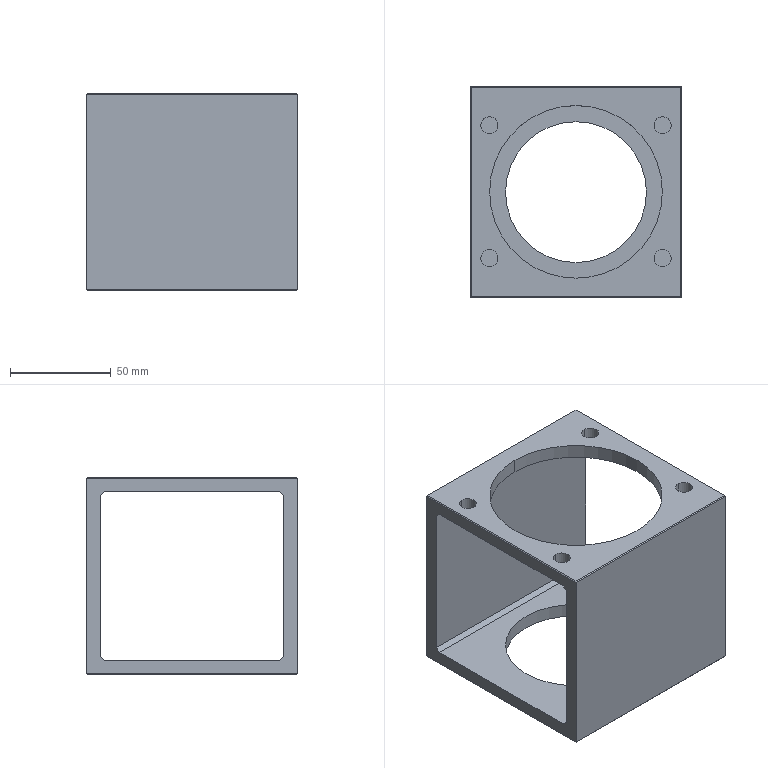Part | Creo | features CURVE 3, DATUM PLANE 3, CHAMFER 2, CUT 2, COORDINATE SYSTEM 1, PROTRUSION 1 | 1 solid | 34 faces | box 105 x 105 x 98 mm | volume 209602 mm3 | plane 22 | cylinder 12 | commonest cylinder face diameters 8.5 x8 70 x2 85.76 x2
STEP:
#1=CARTESIAN_POINT('',(0.,0.,0.));
#2=DIRECTION('',(0.,0.,1.));
#3=DIRECTION('',(1.,0.,0.));
#4=AXIS2_PLACEMENT_3D('',#1,#2,#3);
#5=CARTESIAN_POINT('',(52.,-52.,0.));
#6=VERTEX_POINT('',#5);
#7=CARTESIAN_POINT('',(-52.,-52.,0.));
#8=VERTEX_POINT('',#7);
#9=CARTESIAN_POINT('',(52.,-52.,0.));
#10=DIRECTION('',(-1.,0.,0.));
#11=VECTOR('',#10,104.);
#12=LINE('',#9,#11);
#13=EDGE_CURVE('',#6,#8,#12,.T.);
#14=ORIENTED_EDGE('',*,*,#13,.F.);
#15=CARTESIAN_POINT('',(52.,52.,0.));
#16=VERTEX_POINT('',#15);
#17=CARTESIAN_POINT('',(52.,52.,0.));
#18=DIRECTION('',(0.,-1.,0.));
#19=VECTOR('',#18,104.);
#20=LINE('',#17,#19);
#21=EDGE_CURVE('',#16,#6,#20,.T.);
#22=ORIENTED_EDGE('',*,*,#21,.F.);
#23=CARTESIAN_POINT('',(-52.,52.,0.));
#24=VERTEX_POINT('',#23);
#25=CARTESIAN_POINT('',(-52.,52.,0.));
#26=DIRECTION('',(1.,0.,0.));
#27=VECTOR('',#26,104.);
#28=LINE('',#25,#27);
#29=EDGE_CURVE('',#24,#16,#28,.T.);
#30=ORIENTED_EDGE('',*,*,#29,.F.);
#31=CARTESIAN_POINT('',(-52.,-52.,0.));
#32=DIRECTION('',(0.,1.,0.));
#33=VECTOR('',#32,104.);
#34=LINE('',#31,#33);
#35=EDGE_CURVE('',#8,#24,#34,.T.);
#36=ORIENTED_EDGE('',*,*,#35,.F.);
#37=EDGE_LOOP('',(#14,#22,#30,#36));
#38=FACE_OUTER_BOUND('',#37,.F.);
#39=CARTESIAN_POINT('',(35.,0.,0.));
#40=VERTEX_POINT('',#39);
#41=CARTESIAN_POINT('',(-35.,0.,0.));
#42=VERTEX_POINT('',#41);
#43=CARTESIAN_POINT('',(0.,0.,0.));
#44=DIRECTION('',(0.,0.,-1.));
#45=DIRECTION('',(1.,0.,0.));
#46=AXIS2_PLACEMENT_3D('',#43,#44,#45);
#47=CIRCLE('',#46,35.);
#48=EDGE_CURVE('',#40,#42,#47,.T.);
#49=ORIENTED_EDGE('',*,*,#48,.T.);
#50=CARTESIAN_POINT('',(0.,0.,0.));
#51=DIRECTION('',(0.,0.,-1.));
#52=DIRECTION('',(-1.,0.,0.));
#53=AXIS2_PLACEMENT_3D('',#50,#51,#52);
#54=CIRCLE('',#53,35.);
#55=EDGE_CURVE('',#42,#40,#54,.T.);
#56=ORIENTED_EDGE('',*,*,#55,.T.);
#57=EDGE_LOOP('',(#49,#56));
#58=FACE_BOUND('',#57,.F.);
#59=CARTESIAN_POINT('',(0.,0.,0.));
#60=DIRECTION('',(0.,0.,1.));
#61=DIRECTION('',(1.,0.,0.));
#62=AXIS2_PLACEMENT_3D('',#59,#60,#61);
#63=PLANE('',#62);
#64=ADVANCED_FACE('',(#38,#58),#63,.F.);
#65=CARTESIAN_POINT('',(-35.,0.,7.));
#66=VERTEX_POINT('',#65);
#67=CARTESIAN_POINT('',(35.,0.,7.));
#68=VERTEX_POINT('',#67);
#69=CARTESIAN_POINT('',(0.,0.,7.));
#70=DIRECTION('',(0.,0.,1.));
#71=DIRECTION('',(-1.,0.,0.));
#72=AXIS2_PLACEMENT_3D('',#69,#70,#71);
#73=CIRCLE('',#72,35.);
#74=EDGE_CURVE('',#66,#68,#73,.T.);
#75=ORIENTED_EDGE('',*,*,#74,.F.);
#76=CARTESIAN_POINT('',(-35.,0.,0.));
#77=DIRECTION('',(0.,0.,1.));
#78=VECTOR('',#77,7.);
#79=LINE('',#76,#78);
#80=EDGE_CURVE('',#42,#66,#79,.T.);
#81=ORIENTED_EDGE('',*,*,#80,.F.);
#82=ORIENTED_EDGE('',*,*,#48,.F.);
#83=CARTESIAN_POINT('',(35.,0.,0.));
#84=DIRECTION('',(0.,0.,1.));
#85=VECTOR('',#84,7.);
#86=LINE('',#83,#85);
#87=EDGE_CURVE('',#40,#68,#86,.T.);
#88=ORIENTED_EDGE('',*,*,#87,.T.);
#89=EDGE_LOOP('',(#75,#81,#82,#88));
#90=FACE_OUTER_BOUND('',#89,.F.);
#91=CARTESIAN_POINT('',(0.,0.,0.));
#92=DIRECTION('',(0.,0.,1.));
#93=DIRECTION('',(1.,0.,0.));
#94=AXIS2_PLACEMENT_3D('',#91,#92,#93);
#95=CYLINDRICAL_SURFACE('',#94,35.);
#96=ADVANCED_FACE('',(#90),#95,.F.);
#97=CARTESIAN_POINT('',(52.5,-43.5,7.));
#98=VERTEX_POINT('',#97);
#99=CARTESIAN_POINT('',(-52.5,-43.5,7.));
#100=VERTEX_POINT('',#99);
#101=CARTESIAN_POINT('',(52.5,-43.5,7.));
#102=DIRECTION('',(-1.,0.,0.));
#103=VECTOR('',#102,105.);
#104=LINE('',#101,#103);
#105=EDGE_CURVE('',#98,#100,#104,.T.);
#106=ORIENTED_EDGE('',*,*,#105,.T.);
#107=CARTESIAN_POINT('',(-52.5,43.5,7.));
#108=VERTEX_POINT('',#107);
#109=CARTESIAN_POINT('',(-52.5,-43.5,7.));
#110=DIRECTION('',(0.,1.,0.));
#111=VECTOR('',#110,87.);
#112=LINE('',#109,#111);
#113=EDGE_CURVE('',#100,#108,#112,.T.);
#114=ORIENTED_EDGE('',*,*,#113,.T.);
#115=CARTESIAN_POINT('',(52.5,43.5,7.));
#116=VERTEX_POINT('',#115);
#117=CARTESIAN_POINT('',(52.5,43.5,7.));
#118=DIRECTION('',(-1.,0.,0.));
#119=VECTOR('',#118,105.);
#120=LINE('',#117,#119);
#121=EDGE_CURVE('',#116,#108,#120,.T.);
#122=ORIENTED_EDGE('',*,*,#121,.F.);
#123=CARTESIAN_POINT('',(52.5,-43.5,7.));
#124=DIRECTION('',(0.,1.,0.));
#125=VECTOR('',#124,87.);
#126=LINE('',#123,#125);
#127=EDGE_CURVE('',#98,#116,#126,.T.);
#128=ORIENTED_EDGE('',*,*,#127,.F.);
#129=EDGE_LOOP('',(#106,#114,#122,#128));
#130=FACE_OUTER_BOUND('',#129,.F.);
#131=ORIENTED_EDGE('',*,*,#74,.T.);
#132=CARTESIAN_POINT('',(0.,0.,7.));
#133=DIRECTION('',(0.,0.,1.));
#134=DIRECTION('',(1.,0.,0.));
#135=AXIS2_PLACEMENT_3D('',#132,#133,#134);
#136=CIRCLE('',#135,35.);
#137=EDGE_CURVE('',#68,#66,#136,.T.);
#138=ORIENTED_EDGE('',*,*,#137,.T.);
#139=EDGE_LOOP('',(#131,#138));
#140=FACE_BOUND('',#139,.F.);
#141=CARTESIAN_POINT('',(52.5,-45.5,7.));
#142=DIRECTION('',(0.,0.,-1.));
#143=DIRECTION('',(0.,1.,0.));
#144=AXIS2_PLACEMENT_3D('',#141,#142,#143);
#145=PLANE('',#144);
#146=ADVANCED_FACE('',(#130,#140),#145,.F.);
#147=ORIENTED_EDGE('',*,*,#137,.F.);
#148=ORIENTED_EDGE('',*,*,#87,.F.);
#149=ORIENTED_EDGE('',*,*,#55,.F.);
#150=ORIENTED_EDGE('',*,*,#80,.T.);
#151=EDGE_LOOP('',(#147,#148,#149,#150));
#152=FACE_OUTER_BOUND('',#151,.F.);
#153=CARTESIAN_POINT('',(0.,0.,0.));
#154=DIRECTION('',(0.,0.,1.));
#155=DIRECTION('',(1.,0.,0.));
#156=AXIS2_PLACEMENT_3D('',#153,#154,#155);
#157=CYLINDRICAL_SURFACE('',#156,35.);
#158=ADVANCED_FACE('',(#152),#157,.F.);
#159=ORIENTED_EDGE('',*,*,#105,.F.);
#160=CARTESIAN_POINT('',(52.5,-45.5,9.));
#161=VERTEX_POINT('',#160);
#162=CARTESIAN_POINT('',(52.5,-43.5,7.));
#163=DIRECTION('',(0.,-0.7071,0.7071));
#164=VECTOR('',#163,2.828);
#165=LINE('',#162,#164);
#166=EDGE_CURVE('',#98,#161,#165,.T.);
#167=ORIENTED_EDGE('',*,*,#166,.T.);
#168=CARTESIAN_POINT('',(-52.5,-45.5,9.));
#169=VERTEX_POINT('',#168);
#170=CARTESIAN_POINT('',(52.5,-45.5,9.));
#171=DIRECTION('',(-1.,0.,0.));
#172=VECTOR('',#171,105.);
#173=LINE('',#170,#172);
#174=EDGE_CURVE('',#161,#169,#173,.T.);
#175=ORIENTED_EDGE('',*,*,#174,.T.);
#176=CARTESIAN_POINT('',(-52.5,-45.5,9.));
#177=DIRECTION('',(0.,0.7071,-0.7071));
#178=VECTOR('',#177,2.828);
#179=LINE('',#176,#178);
#180=EDGE_CURVE('',#169,#100,#179,.T.);
#181=ORIENTED_EDGE('',*,*,#180,.T.);
#182=EDGE_LOOP('',(#159,#167,#175,#181));
#183=FACE_OUTER_BOUND('',#182,.F.);
#184=CARTESIAN_POINT('',(0.,-44.5,8.));
#185=DIRECTION('',(0.,0.7071,0.7071));
#186=DIRECTION('',(0.,0.7071,-0.7071));
#187=AXIS2_PLACEMENT_3D('',#184,#185,#186);
#188=PLANE('',#187);
#189=ADVANCED_FACE('',(#183),#188,.T.);
#190=CARTESIAN_POINT('',(52.5,52.5,0.5));
#191=VERTEX_POINT('',#190);
#192=CARTESIAN_POINT('',(52.5,-52.5,0.5));
#193=VERTEX_POINT('',#192);
#194=CARTESIAN_POINT('',(52.5,52.5,0.5));
#195=DIRECTION('',(0.,-1.,0.));
#196=VECTOR('',#195,105.);
#197=LINE('',#194,#196);
#198=EDGE_CURVE('',#191,#193,#197,.T.);
#199=ORIENTED_EDGE('',*,*,#198,.T.);
#200=CARTESIAN_POINT('',(52.5,-52.5,97.5));
#201=VERTEX_POINT('',#200);
#202=CARTESIAN_POINT('',(52.5,-52.5,0.5));
#203=DIRECTION('',(0.,0.,1.));
#204=VECTOR('',#203,97.);
#205=LINE('',#202,#204);
#206=EDGE_CURVE('',#193,#201,#205,.T.);
#207=ORIENTED_EDGE('',*,*,#206,.T.);
#208=CARTESIAN_POINT('',(52.5,52.5,97.5));
#209=VERTEX_POINT('',#208);
#210=CARTESIAN_POINT('',(52.5,-52.5,97.5));
#211=DIRECTION('',(0.,1.,0.));
#212=VECTOR('',#211,105.);
#213=LINE('',#210,#212);
#214=EDGE_CURVE('',#201,#209,#213,.T.);
#215=ORIENTED_EDGE('',*,*,#214,.T.);
#216=CARTESIAN_POINT('',(52.5,52.5,0.5));
#217=DIRECTION('',(0.,0.,1.));
#218=VECTOR('',#217,97.);
#219=LINE('',#216,#218);
#220=EDGE_CURVE('',#191,#209,#219,.T.);
#221=ORIENTED_EDGE('',*,*,#220,.F.);
#222=EDGE_LOOP('',(#199,#207,#215,#221));
#223=FACE_OUTER_BOUND('',#222,.F.);
#224=CARTESIAN_POINT('',(52.5,43.5,91.));
#225=VERTEX_POINT('',#224);
#226=CARTESIAN_POINT('',(52.5,-43.5,91.));
#227=VERTEX_POINT('',#226);
#228=CARTESIAN_POINT('',(52.5,43.5,91.));
#229=DIRECTION('',(0.,-1.,0.));
#230=VECTOR('',#229,87.);
#231=LINE('',#228,#230);
#232=EDGE_CURVE('',#225,#227,#231,.T.);
#233=ORIENTED_EDGE('',*,*,#232,.T.);
#234=CARTESIAN_POINT('',(52.5,-45.5,89.));
#235=VERTEX_POINT('',#234);
#236=CARTESIAN_POINT('',(52.5,-45.5,89.));
#237=DIRECTION('',(0.,0.7071,0.7071));
#238=VECTOR('',#237,2.828);
#239=LINE('',#236,#238);
#240=EDGE_CURVE('',#235,#227,#239,.T.);
#241=ORIENTED_EDGE('',*,*,#240,.F.);
#242=CARTESIAN_POINT('',(52.5,-45.5,89.));
#243=DIRECTION('',(0.,0.,-1.));
#244=VECTOR('',#243,80.);
#245=LINE('',#242,#244);
#246=EDGE_CURVE('',#235,#161,#245,.T.);
#247=ORIENTED_EDGE('',*,*,#246,.T.);
#248=ORIENTED_EDGE('',*,*,#166,.F.);
#249=ORIENTED_EDGE('',*,*,#127,.T.);
#250=CARTESIAN_POINT('',(52.5,45.5,9.));
#251=VERTEX_POINT('',#250);
#252=CARTESIAN_POINT('',(52.5,45.5,9.));
#253=DIRECTION('',(0.,-0.7071,-0.7071));
#254=VECTOR('',#253,2.828);
#255=LINE('',#252,#254);
#256=EDGE_CURVE('',#251,#116,#255,.T.);
#257=ORIENTED_EDGE('',*,*,#256,.F.);
#258=CARTESIAN_POINT('',(52.5,45.5,89.));
#259=VERTEX_POINT('',#258);
#260=CARTESIAN_POINT('',(52.5,45.5,9.));
#261=DIRECTION('',(0.,0.,1.));
#262=VECTOR('',#261,80.);
#263=LINE('',#260,#262);
#264=EDGE_CURVE('',#251,#259,#263,.T.);
#265=ORIENTED_EDGE('',*,*,#264,.T.);
#266=CARTESIAN_POINT('',(52.5,43.5,91.));
#267=DIRECTION('',(0.,0.7071,-0.7071));
#268=VECTOR('',#267,2.828);
#269=LINE('',#266,#268);
#270=EDGE_CURVE('',#225,#259,#269,.T.);
#271=ORIENTED_EDGE('',*,*,#270,.F.);
#272=EDGE_LOOP('',(#233,#241,#247,#248,#249,#257,#265,#271));
#273=FACE_BOUND('',#272,.F.);
#274=CARTESIAN_POINT('',(52.5,-52.5,0.));
#275=DIRECTION('',(1.,0.,0.));
#276=DIRECTION('',(0.,1.,0.));
#277=AXIS2_PLACEMENT_3D('',#274,#275,#276);
#278=PLANE('',#277);
#279=ADVANCED_FACE('',(#223,#273),#278,.T.);
#280=CARTESIAN_POINT('',(-52.5,43.5,91.));
#281=VERTEX_POINT('',#280);
#282=CARTESIAN_POINT('',(52.5,43.5,91.));
#283=DIRECTION('',(-1.,0.,0.));
#284=VECTOR('',#283,105.);
#285=LINE('',#282,#284);
#286=EDGE_CURVE('',#225,#281,#285,.T.);
#287=ORIENTED_EDGE('',*,*,#286,.T.);
#288=CARTESIAN_POINT('',(-52.5,-43.5,91.));
#289=VERTEX_POINT('',#288);
#290=CARTESIAN_POINT('',(-52.5,43.5,91.));
#291=DIRECTION('',(0.,-1.,0.));
#292=VECTOR('',#291,87.);
#293=LINE('',#290,#292);
#294=EDGE_CURVE('',#281,#289,#293,.T.);
#295=ORIENTED_EDGE('',*,*,#294,.T.);
#296=CARTESIAN_POINT('',(52.5,-43.5,91.));
#297=DIRECTION('',(-1.,0.,0.));
#298=VECTOR('',#297,105.);
#299=LINE('',#296,#298);
#300=EDGE_CURVE('',#227,#289,#299,.T.);
#301=ORIENTED_EDGE('',*,*,#300,.F.);
#302=ORIENTED_EDGE('',*,*,#232,.F.);
#303=EDGE_LOOP('',(#287,#295,#301,#302));
#304=FACE_OUTER_BOUND('',#303,.F.);
#305=CARTESIAN_POINT('',(-43.,37.25,91.));
#306=VERTEX_POINT('',#305);
#307=CARTESIAN_POINT('',(-43.,28.75,91.));
#308=VERTEX_POINT('',#307);
#309=CARTESIAN_POINT('',(-43.,33.,91.));
#310=DIRECTION('',(0.,0.,1.));
#311=DIRECTION('',(0.,1.,0.));
#312=AXIS2_PLACEMENT_3D('',#309,#310,#311);
#313=CIRCLE('',#312,4.25);
#314=EDGE_CURVE('',#306,#308,#313,.T.);
#315=ORIENTED_EDGE('',*,*,#314,.F.);
#316=CARTESIAN_POINT('',(-43.,33.,91.));
#317=DIRECTION('',(0.,0.,1.));
#318=DIRECTION('',(0.,-1.,0.));
#319=AXIS2_PLACEMENT_3D('',#316,#317,#318);
#320=CIRCLE('',#319,4.25);
#321=EDGE_CURVE('',#308,#306,#320,.T.);
#322=ORIENTED_EDGE('',*,*,#321,.F.);
#323=EDGE_LOOP('',(#315,#322));
#324=FACE_BOUND('',#323,.F.);
#325=CARTESIAN_POINT('',(-43.,-28.75,91.));
#326=VERTEX_POINT('',#325);
#327=CARTESIAN_POINT('',(-43.,-37.25,91.));
#328=VERTEX_POINT('',#327);
#329=CARTESIAN_POINT('',(-43.,-33.,91.));
#330=DIRECTION('',(0.,0.,1.));
#331=DIRECTION('',(0.,1.,0.));
#332=AXIS2_PLACEMENT_3D('',#329,#330,#331);
#333=CIRCLE('',#332,4.25);
#334=EDGE_CURVE('',#326,#328,#333,.T.);
#335=ORIENTED_EDGE('',*,*,#334,.F.);
#336=CARTESIAN_POINT('',(-43.,-33.,91.));
#337=DIRECTION('',(0.,0.,1.));
#338=DIRECTION('',(0.,-1.,0.));
#339=AXIS2_PLACEMENT_3D('',#336,#337,#338);
#340=CIRCLE('',#339,4.25);
#341=EDGE_CURVE('',#328,#326,#340,.T.);
#342=ORIENTED_EDGE('',*,*,#341,.F.);
#343=EDGE_LOOP('',(#335,#342));
#344=FACE_BOUND('',#343,.F.);
#345=CARTESIAN_POINT('',(43.,-28.75,91.));
#346=VERTEX_POINT('',#345);
#347=CARTESIAN_POINT('',(43.,-37.25,91.));
#348=VERTEX_POINT('',#347);
#349=CARTESIAN_POINT('',(43.,-33.,91.));
#350=DIRECTION('',(0.,0.,1.));
#351=DIRECTION('',(0.,1.,0.));
#352=AXIS2_PLACEMENT_3D('',#349,#350,#351);
#353=CIRCLE('',#352,4.25);
#354=EDGE_CURVE('',#346,#348,#353,.T.);
#355=ORIENTED_EDGE('',*,*,#354,.F.);
#356=CARTESIAN_POINT('',(43.,-33.,91.));
#357=DIRECTION('',(0.,0.,1.));
#358=DIRECTION('',(0.,-1.,0.));
#359=AXIS2_PLACEMENT_3D('',#356,#357,#358);
#360=CIRCLE('',#359,4.25);
#361=EDGE_CURVE('',#348,#346,#360,.T.);
#362=ORIENTED_EDGE('',*,*,#361,.F.);
#363=EDGE_LOOP('',(#355,#362));
#364=FACE_BOUND('',#363,.F.);
#365=CARTESIAN_POINT('',(43.,37.25,91.));
#366=VERTEX_POINT('',#365);
#367=CARTESIAN_POINT('',(43.,28.75,91.));
#368=VERTEX_POINT('',#367);
#369=CARTESIAN_POINT('',(43.,33.,91.));
#370=DIRECTION('',(0.,0.,1.));
#371=DIRECTION('',(0.,1.,0.));
#372=AXIS2_PLACEMENT_3D('',#369,#370,#371);
#373=CIRCLE('',#372,4.25);
#374=EDGE_CURVE('',#366,#368,#373,.T.);
#375=ORIENTED_EDGE('',*,*,#374,.F.);
#376=CARTESIAN_POINT('',(43.,33.,91.));
#377=DIRECTION('',(0.,0.,1.));
#378=DIRECTION('',(0.,-1.,0.));
#379=AXIS2_PLACEMENT_3D('',#376,#377,#378);
#380=CIRCLE('',#379,4.25);
#381=EDGE_CURVE('',#368,#366,#380,.T.);
#382=ORIENTED_EDGE('',*,*,#381,.F.);
#383=EDGE_LOOP('',(#375,#382));
#384=FACE_BOUND('',#383,.F.);
#385=CARTESIAN_POINT('',(0.,42.88,91.));
#386=VERTEX_POINT('',#385);
#387=CARTESIAN_POINT('',(0.,-42.88,91.));
#388=VERTEX_POINT('',#387);
#389=CARTESIAN_POINT('',(0.,0.,91.));
#390=DIRECTION('',(0.,0.,1.));
#391=DIRECTION('',(0.,1.,0.));
#392=AXIS2_PLACEMENT_3D('',#389,#390,#391);
#393=CIRCLE('',#392,42.88);
#394=EDGE_CURVE('',#386,#388,#393,.T.);
#395=ORIENTED_EDGE('',*,*,#394,.F.);
#396=CARTESIAN_POINT('',(0.,0.,91.));
#397=DIRECTION('',(0.,0.,1.));
#398=DIRECTION('',(0.,-1.,0.));
#399=AXIS2_PLACEMENT_3D('',#396,#397,#398);
#400=CIRCLE('',#399,42.88);
#401=EDGE_CURVE('',#388,#386,#400,.T.);
#402=ORIENTED_EDGE('',*,*,#401,.F.);
#403=EDGE_LOOP('',(#395,#402));
#404=FACE_BOUND('',#403,.F.);
#405=CARTESIAN_POINT('',(52.5,45.5,91.));
#406=DIRECTION('',(0.,0.,1.));
#407=DIRECTION('',(0.,-1.,0.));
#408=AXIS2_PLACEMENT_3D('',#405,#406,#407);
#409=PLANE('',#408);
#410=ADVANCED_FACE('',(#304,#324,#344,#364,#384,#404),#409,.F.);
#411=CARTESIAN_POINT('',(0.,42.88,98.));
#412=VERTEX_POINT('',#411);
#413=CARTESIAN_POINT('',(0.,-42.88,98.));
#414=VERTEX_POINT('',#413);
#415=CARTESIAN_POINT('',(0.,0.,98.));
#416=DIRECTION('',(0.,0.,1.));
#417=DIRECTION('',(0.,1.,0.));
#418=AXIS2_PLACEMENT_3D('',#415,#416,#417);
#419=CIRCLE('',#418,42.88);
#420=EDGE_CURVE('',#412,#414,#419,.T.);
#421=ORIENTED_EDGE('',*,*,#420,.F.);
#422=CARTESIAN_POINT('',(0.,42.88,98.));
#423=DIRECTION('',(0.,0.,-1.));
#424=VECTOR('',#423,7.);
#425=LINE('',#422,#424);
#426=EDGE_CURVE('',#412,#386,#425,.T.);
#427=ORIENTED_EDGE('',*,*,#426,.T.);
#428=ORIENTED_EDGE('',*,*,#394,.T.);
#429=CARTESIAN_POINT('',(0.,-42.88,98.));
#430=DIRECTION('',(0.,0.,-1.));
#431=VECTOR('',#430,7.);
#432=LINE('',#429,#431);
#433=EDGE_CURVE('',#414,#388,#432,.T.);
#434=ORIENTED_EDGE('',*,*,#433,.F.);
#435=EDGE_LOOP('',(#421,#427,#428,#434));
#436=FACE_OUTER_BOUND('',#435,.F.);
#437=CARTESIAN_POINT('',(0.,0.,98.));
#438=DIRECTION('',(0.,0.,1.));
#439=DIRECTION('',(0.,1.,0.));
#440=AXIS2_PLACEMENT_3D('',#437,#438,#439);
#441=CYLINDRICAL_SURFACE('',#440,42.88);
#442=ADVANCED_FACE('',(#436),#441,.F.);
#443=CARTESIAN_POINT('',(-52.,52.,98.));
#444=VERTEX_POINT('',#443);
#445=CARTESIAN_POINT('',(-52.,-52.,98.));
#446=VERTEX_POINT('',#445);
#447=CARTESIAN_POINT('',(-52.,52.,98.));
#448=DIRECTION('',(0.,-1.,0.));
#449=VECTOR('',#448,104.);
#450=LINE('',#447,#449);
#451=EDGE_CURVE('',#444,#446,#450,.T.);
#452=ORIENTED_EDGE('',*,*,#451,.F.);
#453=CARTESIAN_POINT('',(52.,52.,98.));
#454=VERTEX_POINT('',#453);
#455=CARTESIAN_POINT('',(52.,52.,98.));
#456=DIRECTION('',(-1.,0.,0.));
#457=VECTOR('',#456,104.);
#458=LINE('',#455,#457);
#459=EDGE_CURVE('',#454,#444,#458,.T.);
#460=ORIENTED_EDGE('',*,*,#459,.F.);
#461=CARTESIAN_POINT('',(52.,-52.,98.));
#462=VERTEX_POINT('',#461);
#463=CARTESIAN_POINT('',(52.,-52.,98.));
#464=DIRECTION('',(0.,1.,0.));
#465=VECTOR('',#464,104.);
#466=LINE('',#463,#465);
#467=EDGE_CURVE('',#462,#454,#466,.T.);
#468=ORIENTED_EDGE('',*,*,#467,.F.);
#469=CARTESIAN_POINT('',(-52.,-52.,98.));
#470=DIRECTION('',(1.,0.,0.));
#471=VECTOR('',#470,104.);
#472=LINE('',#469,#471);
#473=EDGE_CURVE('',#446,#462,#472,.T.);
#474=ORIENTED_EDGE('',*,*,#473,.F.);
#475=EDGE_LOOP('',(#452,#460,#468,#474));
#476=FACE_OUTER_BOUND('',#475,.F.);
#477=CARTESIAN_POINT('',(-43.,37.25,98.));
#478=VERTEX_POINT('',#477);
#479=CARTESIAN_POINT('',(-43.,28.75,98.));
#480=VERTEX_POINT('',#479);
#481=CARTESIAN_POINT('',(-43.,33.,98.));
#482=DIRECTION('',(0.,0.,1.));
#483=DIRECTION('',(0.,1.,0.));
#484=AXIS2_PLACEMENT_3D('',#481,#482,#483);
#485=CIRCLE('',#484,4.25);
#486=EDGE_CURVE('',#478,#480,#485,.T.);
#487=ORIENTED_EDGE('',*,*,#486,.T.);
#488=CARTESIAN_POINT('',(-43.,33.,98.));
#489=DIRECTION('',(0.,0.,1.));
#490=DIRECTION('',(0.,-1.,0.));
#491=AXIS2_PLACEMENT_3D('',#488,#489,#490);
#492=CIRCLE('',#491,4.25);
#493=EDGE_CURVE('',#480,#478,#492,.T.);
#494=ORIENTED_EDGE('',*,*,#493,.T.);
#495=EDGE_LOOP('',(#487,#494));
#496=FACE_BOUND('',#495,.F.);
#497=CARTESIAN_POINT('',(-43.,-28.75,98.));
#498=VERTEX_POINT('',#497);
#499=CARTESIAN_POINT('',(-43.,-37.25,98.));
#500=VERTEX_POINT('',#499);
#501=CARTESIAN_POINT('',(-43.,-33.,98.));
#502=DIRECTION('',(0.,0.,1.));
#503=DIRECTION('',(0.,1.,0.));
#504=AXIS2_PLACEMENT_3D('',#501,#502,#503);
#505=CIRCLE('',#504,4.25);
#506=EDGE_CURVE('',#498,#500,#505,.T.);
#507=ORIENTED_EDGE('',*,*,#506,.T.);
#508=CARTESIAN_POINT('',(-43.,-33.,98.));
#509=DIRECTION('',(0.,0.,1.));
#510=DIRECTION('',(0.,-1.,0.));
#511=AXIS2_PLACEMENT_3D('',#508,#509,#510);
#512=CIRCLE('',#511,4.25);
#513=EDGE_CURVE('',#500,#498,#512,.T.);
#514=ORIENTED_EDGE('',*,*,#513,.T.);
#515=EDGE_LOOP('',(#507,#514));
#516=FACE_BOUND('',#515,.F.);
#517=CARTESIAN_POINT('',(43.,-28.75,98.));
#518=VERTEX_POINT('',#517);
#519=CARTESIAN_POINT('',(43.,-37.25,98.));
#520=VERTEX_POINT('',#519);
#521=CARTESIAN_POINT('',(43.,-33.,98.));
#522=DIRECTION('',(0.,0.,1.));
#523=DIRECTION('',(0.,1.,0.));
#524=AXIS2_PLACEMENT_3D('',#521,#522,#523);
#525=CIRCLE('',#524,4.25);
#526=EDGE_CURVE('',#518,#520,#525,.T.);
#527=ORIENTED_EDGE('',*,*,#526,.T.);
#528=CARTESIAN_POINT('',(43.,-33.,98.));
#529=DIRECTION('',(0.,0.,1.));
#530=DIRECTION('',(0.,-1.,0.));
#531=AXIS2_PLACEMENT_3D('',#528,#529,#530);
#532=CIRCLE('',#531,4.25);
#533=EDGE_CURVE('',#520,#518,#532,.T.);
#534=ORIENTED_EDGE('',*,*,#533,.T.);
#535=EDGE_LOOP('',(#527,#534));
#536=FACE_BOUND('',#535,.F.);
#537=CARTESIAN_POINT('',(43.,37.25,98.));
#538=VERTEX_POINT('',#537);
#539=CARTESIAN_POINT('',(43.,28.75,98.));
#540=VERTEX_POINT('',#539);
#541=CARTESIAN_POINT('',(43.,33.,98.));
#542=DIRECTION('',(0.,0.,1.));
#543=DIRECTION('',(0.,1.,0.));
#544=AXIS2_PLACEMENT_3D('',#541,#542,#543);
#545=CIRCLE('',#544,4.25);
#546=EDGE_CURVE('',#538,#540,#545,.T.);
#547=ORIENTED_EDGE('',*,*,#546,.T.);
#548=CARTESIAN_POINT('',(43.,33.,98.));
#549=DIRECTION('',(0.,0.,1.));
#550=DIRECTION('',(0.,-1.,0.));
#551=AXIS2_PLACEMENT_3D('',#548,#549,#550);
#552=CIRCLE('',#551,4.25);
#553=EDGE_CURVE('',#540,#538,#552,.T.);
#554=ORIENTED_EDGE('',*,*,#553,.T.);
#555=EDGE_LOOP('',(#547,#554));
#556=FACE_BOUND('',#555,.F.);
#557=ORIENTED_EDGE('',*,*,#420,.T.);
#558=CARTESIAN_POINT('',(0.,0.,98.));
#559=DIRECTION('',(0.,0.,1.));
#560=DIRECTION('',(0.,-1.,0.));
#561=AXIS2_PLACEMENT_3D('',#558,#559,#560);
#562=CIRCLE('',#561,42.88);
#563=EDGE_CURVE('',#414,#412,#562,.T.);
#564=ORIENTED_EDGE('',*,*,#563,.T.);
#565=EDGE_LOOP('',(#557,#564));
#566=FACE_BOUND('',#565,.F.);
#567=CARTESIAN_POINT('',(0.,0.,98.));
#568=DIRECTION('',(0.,0.,1.));
#569=DIRECTION('',(1.,0.,0.));
#570=AXIS2_PLACEMENT_3D('',#567,#568,#569);
#571=PLANE('',#570);
#572=ADVANCED_FACE('',(#476,#496,#516,#536,#556,#566),#571,.T.);
#573=ORIENTED_EDGE('',*,*,#563,.F.);
#574=ORIENTED_EDGE('',*,*,#433,.T.);
#575=ORIENTED_EDGE('',*,*,#401,.T.);
#576=ORIENTED_EDGE('',*,*,#426,.F.);
#577=EDGE_LOOP('',(#573,#574,#575,#576));
#578=FACE_OUTER_BOUND('',#577,.F.);
#579=CARTESIAN_POINT('',(0.,0.,98.));
#580=DIRECTION('',(0.,0.,1.));
#581=DIRECTION('',(0.,1.,0.));
#582=AXIS2_PLACEMENT_3D('',#579,#580,#581);
#583=CYLINDRICAL_SURFACE('',#582,42.88);
#584=ADVANCED_FACE('',(#578),#583,.F.);
#585=ORIENTED_EDGE('',*,*,#486,.F.);
#586=CARTESIAN_POINT('',(-43.,37.25,98.));
#587=DIRECTION('',(0.,0.,-1.));
#588=VECTOR('',#587,7.);
#589=LINE('',#586,#588);
#590=EDGE_CURVE('',#478,#306,#589,.T.);
#591=ORIENTED_EDGE('',*,*,#590,.T.);
#592=ORIENTED_EDGE('',*,*,#314,.T.);
#593=CARTESIAN_POINT('',(-43.,28.75,98.));
#594=DIRECTION('',(0.,0.,-1.));
#595=VECTOR('',#594,7.);
#596=LINE('',#593,#595);
#597=EDGE_CURVE('',#480,#308,#596,.T.);
#598=ORIENTED_EDGE('',*,*,#597,.F.);
#599=EDGE_LOOP('',(#585,#591,#592,#598));
#600=FACE_OUTER_BOUND('',#599,.F.);
#601=CARTESIAN_POINT('',(-43.,33.,98.));
#602=DIRECTION('',(0.,0.,1.));
#603=DIRECTION('',(0.,1.,0.));
#604=AXIS2_PLACEMENT_3D('',#601,#602,#603);
#605=CYLINDRICAL_SURFACE('',#604,4.25);
#606=ADVANCED_FACE('',(#600),#605,.F.);
#607=ORIENTED_EDGE('',*,*,#493,.F.);
#608=ORIENTED_EDGE('',*,*,#597,.T.);
#609=ORIENTED_EDGE('',*,*,#321,.T.);
#610=ORIENTED_EDGE('',*,*,#590,.F.);
#611=EDGE_LOOP('',(#607,#608,#609,#610));
#612=FACE_OUTER_BOUND('',#611,.F.);
#613=CARTESIAN_POINT('',(-43.,33.,98.));
#614=DIRECTION('',(0.,0.,1.));
#615=DIRECTION('',(0.,1.,0.));
#616=AXIS2_PLACEMENT_3D('',#613,#614,#615);
#617=CYLINDRICAL_SURFACE('',#616,4.25);
#618=ADVANCED_FACE('',(#612),#617,.F.);
#619=ORIENTED_EDGE('',*,*,#506,.F.);
#620=CARTESIAN_POINT('',(-43.,-28.75,98.));
#621=DIRECTION('',(0.,0.,-1.));
#622=VECTOR('',#621,7.);
#623=LINE('',#620,#622);
#624=EDGE_CURVE('',#498,#326,#623,.T.);
#625=ORIENTED_EDGE('',*,*,#624,.T.);
#626=ORIENTED_EDGE('',*,*,#334,.T.);
#627=CARTESIAN_POINT('',(-43.,-37.25,98.));
#628=DIRECTION('',(0.,0.,-1.));
#629=VECTOR('',#628,7.);
#630=LINE('',#627,#629);
#631=EDGE_CURVE('',#500,#328,#630,.T.);
#632=ORIENTED_EDGE('',*,*,#631,.F.);
#633=EDGE_LOOP('',(#619,#625,#626,#632));
#634=FACE_OUTER_BOUND('',#633,.F.);
#635=CARTESIAN_POINT('',(-43.,-33.,98.));
#636=DIRECTION('',(0.,0.,1.));
#637=DIRECTION('',(0.,1.,0.));
#638=AXIS2_PLACEMENT_3D('',#635,#636,#637);
#639=CYLINDRICAL_SURFACE('',#638,4.25);
#640=ADVANCED_FACE('',(#634),#639,.F.);
#641=ORIENTED_EDGE('',*,*,#513,.F.);
#642=ORIENTED_EDGE('',*,*,#631,.T.);
#643=ORIENTED_EDGE('',*,*,#341,.T.);
#644=ORIENTED_EDGE('',*,*,#624,.F.);
#645=EDGE_LOOP('',(#641,#642,#643,#644));
#646=FACE_OUTER_BOUND('',#645,.F.);
#647=CARTESIAN_POINT('',(-43.,-33.,98.));
#648=DIRECTION('',(0.,0.,1.));
#649=DIRECTION('',(0.,1.,0.));
#650=AXIS2_PLACEMENT_3D('',#647,#648,#649);
#651=CYLINDRICAL_SURFACE('',#650,4.25);
#652=ADVANCED_FACE('',(#646),#651,.F.);
#653=ORIENTED_EDGE('',*,*,#526,.F.);
#654=CARTESIAN_POINT('',(43.,-28.75,98.));
#655=DIRECTION('',(0.,0.,-1.));
#656=VECTOR('',#655,7.);
#657=LINE('',#654,#656);
#658=EDGE_CURVE('',#518,#346,#657,.T.);
#659=ORIENTED_EDGE('',*,*,#658,.T.);
#660=ORIENTED_EDGE('',*,*,#354,.T.);
#661=CARTESIAN_POINT('',(43.,-37.25,98.));
#662=DIRECTION('',(0.,0.,-1.));
#663=VECTOR('',#662,7.);
#664=LINE('',#661,#663);
#665=EDGE_CURVE('',#520,#348,#664,.T.);
#666=ORIENTED_EDGE('',*,*,#665,.F.);
#667=EDGE_LOOP('',(#653,#659,#660,#666));
#668=FACE_OUTER_BOUND('',#667,.F.);
#669=CARTESIAN_POINT('',(43.,-33.,98.));
#670=DIRECTION('',(0.,0.,1.));
#671=DIRECTION('',(0.,1.,0.));
#672=AXIS2_PLACEMENT_3D('',#669,#670,#671);
#673=CYLINDRICAL_SURFACE('',#672,4.25);
#674=ADVANCED_FACE('',(#668),#673,.F.);
#675=ORIENTED_EDGE('',*,*,#533,.F.);
#676=ORIENTED_EDGE('',*,*,#665,.T.);
#677=ORIENTED_EDGE('',*,*,#361,.T.);
#678=ORIENTED_EDGE('',*,*,#658,.F.);
#679=EDGE_LOOP('',(#675,#676,#677,#678));
#680=FACE_OUTER_BOUND('',#679,.F.);
#681=CARTESIAN_POINT('',(43.,-33.,98.));
#682=DIRECTION('',(0.,0.,1.));
#683=DIRECTION('',(0.,1.,0.));
#684=AXIS2_PLACEMENT_3D('',#681,#682,#683);
#685=CYLINDRICAL_SURFACE('',#684,4.25);
#686=ADVANCED_FACE('',(#680),#685,.F.);
#687=ORIENTED_EDGE('',*,*,#546,.F.);
#688=CARTESIAN_POINT('',(43.,37.25,98.));
#689=DIRECTION('',(0.,0.,-1.));
#690=VECTOR('',#689,7.);
#691=LINE('',#688,#690);
#692=EDGE_CURVE('',#538,#366,#691,.T.);
#693=ORIENTED_EDGE('',*,*,#692,.T.);
#694=ORIENTED_EDGE('',*,*,#374,.T.);
#695=CARTESIAN_POINT('',(43.,28.75,98.));
#696=DIRECTION('',(0.,0.,-1.));
#697=VECTOR('',#696,7.);
#698=LINE('',#695,#697);
#699=EDGE_CURVE('',#540,#368,#698,.T.);
#700=ORIENTED_EDGE('',*,*,#699,.F.);
#701=EDGE_LOOP('',(#687,#693,#694,#700));
#702=FACE_OUTER_BOUND('',#701,.F.);
#703=CARTESIAN_POINT('',(43.,33.,98.));
#704=DIRECTION('',(0.,0.,1.));
#705=DIRECTION('',(0.,1.,0.));
#706=AXIS2_PLACEMENT_3D('',#703,#704,#705);
#707=CYLINDRICAL_SURFACE('',#706,4.25);
#708=ADVANCED_FACE('',(#702),#707,.F.);
#709=ORIENTED_EDGE('',*,*,#553,.F.);
#710=ORIENTED_EDGE('',*,*,#699,.T.);
#711=ORIENTED_EDGE('',*,*,#381,.T.);
#712=ORIENTED_EDGE('',*,*,#692,.F.);
#713=EDGE_LOOP('',(#709,#710,#711,#712));
#714=FACE_OUTER_BOUND('',#713,.F.);
#715=CARTESIAN_POINT('',(43.,33.,98.));
#716=DIRECTION('',(0.,0.,1.));
#717=DIRECTION('',(0.,1.,0.));
#718=AXIS2_PLACEMENT_3D('',#715,#716,#717);
#719=CYLINDRICAL_SURFACE('',#718,4.25);
#720=ADVANCED_FACE('',(#714),#719,.F.);
#721=CARTESIAN_POINT('',(-52.5,52.5,97.5));
#722=VERTEX_POINT('',#721);
#723=CARTESIAN_POINT('',(-52.5,-52.5,97.5));
#724=VERTEX_POINT('',#723);
#725=CARTESIAN_POINT('',(-52.5,52.5,97.5));
#726=DIRECTION('',(0.,-1.,0.));
#727=VECTOR('',#726,105.);
#728=LINE('',#725,#727);
#729=EDGE_CURVE('',#722,#724,#728,.T.);
#730=ORIENTED_EDGE('',*,*,#729,.F.);
#731=CARTESIAN_POINT('',(-52.5,52.5,97.5));
#732=DIRECTION('',(0.5774,-0.5774,0.5774));
#733=VECTOR('',#732,0.866);
#734=LINE('',#731,#733);
#735=EDGE_CURVE('',#722,#444,#734,.T.);
#736=ORIENTED_EDGE('',*,*,#735,.T.);
#737=ORIENTED_EDGE('',*,*,#451,.T.);
#738=CARTESIAN_POINT('',(-52.5,-52.5,97.5));
#739=DIRECTION('',(0.5774,0.5774,0.5774));
#740=VECTOR('',#739,0.866);
#741=LINE('',#738,#740);
#742=EDGE_CURVE('',#724,#446,#741,.T.);
#743=ORIENTED_EDGE('',*,*,#742,.F.);
#744=EDGE_LOOP('',(#730,#736,#737,#743));
#745=FACE_OUTER_BOUND('',#744,.F.);
#746=CARTESIAN_POINT('',(-52.25,0.,97.75));
#747=DIRECTION('',(-0.7071,0.,0.7071));
#748=DIRECTION('',(-0.7071,0.,-0.7071));
#749=AXIS2_PLACEMENT_3D('',#746,#747,#748);
#750=PLANE('',#749);
#751=ADVANCED_FACE('',(#745),#750,.T.);
#752=CARTESIAN_POINT('',(-52.5,-52.5,0.5));
#753=VERTEX_POINT('',#752);
#754=CARTESIAN_POINT('',(-52.5,52.5,0.5));
#755=VERTEX_POINT('',#754);
#756=CARTESIAN_POINT('',(-52.5,-52.5,0.5));
#757=DIRECTION('',(0.,1.,0.));
#758=VECTOR('',#757,105.);
#759=LINE('',#756,#758);
#760=EDGE_CURVE('',#753,#755,#759,.T.);
#761=ORIENTED_EDGE('',*,*,#760,.T.);
#762=CARTESIAN_POINT('',(-52.5,52.5,0.5));
#763=DIRECTION('',(0.,0.,1.));
#764=VECTOR('',#763,97.);
#765=LINE('',#762,#764);
#766=EDGE_CURVE('',#755,#722,#765,.T.);
#767=ORIENTED_EDGE('',*,*,#766,.T.);
#768=ORIENTED_EDGE('',*,*,#729,.T.);
#769=CARTESIAN_POINT('',(-52.5,-52.5,0.5));
#770=DIRECTION('',(0.,0.,1.));
#771=VECTOR('',#770,97.);
#772=LINE('',#769,#771);
#773=EDGE_CURVE('',#753,#724,#772,.T.);
#774=ORIENTED_EDGE('',*,*,#773,.F.);
#775=EDGE_LOOP('',(#761,#767,#768,#774));
#776=FACE_OUTER_BOUND('',#775,.F.);
#777=CARTESIAN_POINT('',(-52.5,-45.5,89.));
#778=VERTEX_POINT('',#777);
#779=CARTESIAN_POINT('',(-52.5,-45.5,89.));
#780=DIRECTION('',(0.,0.,-1.));
#781=VECTOR('',#780,80.);
#782=LINE('',#779,#781);
#783=EDGE_CURVE('',#778,#169,#782,.T.);
#784=ORIENTED_EDGE('',*,*,#783,.F.);
#785=CARTESIAN_POINT('',(-52.5,-43.5,91.));
#786=DIRECTION('',(0.,-0.7071,-0.7071));
#787=VECTOR('',#786,2.828);
#788=LINE('',#785,#787);
#789=EDGE_CURVE('',#289,#778,#788,.T.);
#790=ORIENTED_EDGE('',*,*,#789,.F.);
#791=ORIENTED_EDGE('',*,*,#294,.F.);
#792=CARTESIAN_POINT('',(-52.5,45.5,89.));
#793=VERTEX_POINT('',#792);
#794=CARTESIAN_POINT('',(-52.5,45.5,89.));
#795=DIRECTION('',(0.,-0.7071,0.7071));
#796=VECTOR('',#795,2.828);
#797=LINE('',#794,#796);
#798=EDGE_CURVE('',#793,#281,#797,.T.);
#799=ORIENTED_EDGE('',*,*,#798,.F.);
#800=CARTESIAN_POINT('',(-52.5,45.5,9.));
#801=VERTEX_POINT('',#800);
#802=CARTESIAN_POINT('',(-52.5,45.5,9.));
#803=DIRECTION('',(0.,0.,1.));
#804=VECTOR('',#803,80.);
#805=LINE('',#802,#804);
#806=EDGE_CURVE('',#801,#793,#805,.T.);
#807=ORIENTED_EDGE('',*,*,#806,.F.);
#808=CARTESIAN_POINT('',(-52.5,43.5,7.));
#809=DIRECTION('',(0.,0.7071,0.7071));
#810=VECTOR('',#809,2.828);
#811=LINE('',#808,#810);
#812=EDGE_CURVE('',#108,#801,#811,.T.);
#813=ORIENTED_EDGE('',*,*,#812,.F.);
#814=ORIENTED_EDGE('',*,*,#113,.F.);
#815=ORIENTED_EDGE('',*,*,#180,.F.);
#816=EDGE_LOOP('',(#784,#790,#791,#799,#807,#813,#814,#815));
#817=FACE_BOUND('',#816,.F.);
#818=CARTESIAN_POINT('',(-52.5,52.5,0.));
#819=DIRECTION('',(-1.,0.,0.));
#820=DIRECTION('',(0.,-1.,0.));
#821=AXIS2_PLACEMENT_3D('',#818,#819,#820);
#822=PLANE('',#821);
#823=ADVANCED_FACE('',(#776,#817),#822,.T.);
#824=CARTESIAN_POINT('',(52.5,-45.5,89.));
#825=DIRECTION('',(-1.,0.,0.));
#826=VECTOR('',#825,105.);
#827=LINE('',#824,#826);
#828=EDGE_CURVE('',#235,#778,#827,.T.);
#829=ORIENTED_EDGE('',*,*,#828,.T.);
#830=ORIENTED_EDGE('',*,*,#783,.T.);
#831=ORIENTED_EDGE('',*,*,#174,.F.);
#832=ORIENTED_EDGE('',*,*,#246,.F.);
#833=EDGE_LOOP('',(#829,#830,#831,#832));
#834=FACE_OUTER_BOUND('',#833,.F.);
#835=CARTESIAN_POINT('',(52.5,-45.5,91.));
#836=DIRECTION('',(0.,-1.,0.));
#837=DIRECTION('',(0.,0.,-1.));
#838=AXIS2_PLACEMENT_3D('',#835,#836,#837);
#839=PLANE('',#838);
#840=ADVANCED_FACE('',(#834),#839,.F.);
#841=ORIENTED_EDGE('',*,*,#828,.F.);
#842=ORIENTED_EDGE('',*,*,#240,.T.);
#843=ORIENTED_EDGE('',*,*,#300,.T.);
#844=ORIENTED_EDGE('',*,*,#789,.T.);
#845=EDGE_LOOP('',(#841,#842,#843,#844));
#846=FACE_OUTER_BOUND('',#845,.F.);
#847=CARTESIAN_POINT('',(0.,-44.5,90.));
#848=DIRECTION('',(0.,0.7071,-0.7071));
#849=DIRECTION('',(0.,-0.7071,-0.7071));
#850=AXIS2_PLACEMENT_3D('',#847,#848,#849);
#851=PLANE('',#850);
#852=ADVANCED_FACE('',(#846),#851,.T.);
#853=ORIENTED_EDGE('',*,*,#286,.F.);
#854=ORIENTED_EDGE('',*,*,#270,.T.);
#855=CARTESIAN_POINT('',(52.5,45.5,89.));
#856=DIRECTION('',(-1.,0.,0.));
#857=VECTOR('',#856,105.);
#858=LINE('',#855,#857);
#859=EDGE_CURVE('',#259,#793,#858,.T.);
#860=ORIENTED_EDGE('',*,*,#859,.T.);
#861=ORIENTED_EDGE('',*,*,#798,.T.);
#862=EDGE_LOOP('',(#853,#854,#860,#861));
#863=FACE_OUTER_BOUND('',#862,.F.);
#864=CARTESIAN_POINT('',(0.,44.5,90.));
#865=DIRECTION('',(0.,-0.7071,-0.7071));
#866=DIRECTION('',(0.,-0.7071,0.7071));
#867=AXIS2_PLACEMENT_3D('',#864,#865,#866);
#868=PLANE('',#867);
#869=ADVANCED_FACE('',(#863),#868,.T.);
#870=ORIENTED_EDGE('',*,*,#859,.F.);
#871=ORIENTED_EDGE('',*,*,#264,.F.);
#872=CARTESIAN_POINT('',(52.5,45.5,9.));
#873=DIRECTION('',(-1.,0.,0.));
#874=VECTOR('',#873,105.);
#875=LINE('',#872,#874);
#876=EDGE_CURVE('',#251,#801,#875,.T.);
#877=ORIENTED_EDGE('',*,*,#876,.T.);
#878=ORIENTED_EDGE('',*,*,#806,.T.);
#879=EDGE_LOOP('',(#870,#871,#877,#878));
#880=FACE_OUTER_BOUND('',#879,.F.);
#881=CARTESIAN_POINT('',(52.5,45.5,7.));
#882=DIRECTION('',(0.,1.,0.));
#883=DIRECTION('',(0.,0.,1.));
#884=AXIS2_PLACEMENT_3D('',#881,#882,#883);
#885=PLANE('',#884);
#886=ADVANCED_FACE('',(#880),#885,.F.);
#887=ORIENTED_EDGE('',*,*,#876,.F.);
#888=ORIENTED_EDGE('',*,*,#256,.T.);
#889=ORIENTED_EDGE('',*,*,#121,.T.);
#890=ORIENTED_EDGE('',*,*,#812,.T.);
#891=EDGE_LOOP('',(#887,#888,#889,#890));
#892=FACE_OUTER_BOUND('',#891,.F.);
#893=CARTESIAN_POINT('',(0.,44.5,8.));
#894=DIRECTION('',(0.,-0.7071,0.7071));
#895=DIRECTION('',(0.,0.7071,0.7071));
#896=AXIS2_PLACEMENT_3D('',#893,#894,#895);
#897=PLANE('',#896);
#898=ADVANCED_FACE('',(#892),#897,.T.);
#899=ORIENTED_EDGE('',*,*,#35,.T.);
#900=CARTESIAN_POINT('',(-52.5,52.5,0.5));
#901=DIRECTION('',(0.5774,-0.5774,-0.5774));
#902=VECTOR('',#901,0.866);
#903=LINE('',#900,#902);
#904=EDGE_CURVE('',#755,#24,#903,.T.);
#905=ORIENTED_EDGE('',*,*,#904,.F.);
#906=ORIENTED_EDGE('',*,*,#760,.F.);
#907=CARTESIAN_POINT('',(-52.5,-52.5,0.5));
#908=DIRECTION('',(0.5774,0.5774,-0.5774));
#909=VECTOR('',#908,0.866);
#910=LINE('',#907,#909);
#911=EDGE_CURVE('',#753,#8,#910,.T.);
#912=ORIENTED_EDGE('',*,*,#911,.T.);
#913=EDGE_LOOP('',(#899,#905,#906,#912));
#914=FACE_OUTER_BOUND('',#913,.F.);
#915=CARTESIAN_POINT('',(-52.25,0.,0.25));
#916=DIRECTION('',(-0.7071,0.,-0.7071));
#917=DIRECTION('',(-0.7071,0.,0.7071));
#918=AXIS2_PLACEMENT_3D('',#915,#916,#917);
#919=PLANE('',#918);
#920=ADVANCED_FACE('',(#914),#919,.T.);
#921=ORIENTED_EDGE('',*,*,#29,.T.);
#922=CARTESIAN_POINT('',(52.5,52.5,0.5));
#923=DIRECTION('',(-0.5774,-0.5774,-0.5774));
#924=VECTOR('',#923,0.866);
#925=LINE('',#922,#924);
#926=EDGE_CURVE('',#191,#16,#925,.T.);
#927=ORIENTED_EDGE('',*,*,#926,.F.);
#928=CARTESIAN_POINT('',(-52.5,52.5,0.5));
#929=DIRECTION('',(1.,0.,0.));
#930=VECTOR('',#929,105.);
#931=LINE('',#928,#930);
#932=EDGE_CURVE('',#755,#191,#931,.T.);
#933=ORIENTED_EDGE('',*,*,#932,.F.);
#934=ORIENTED_EDGE('',*,*,#904,.T.);
#935=EDGE_LOOP('',(#921,#927,#933,#934));
#936=FACE_OUTER_BOUND('',#935,.F.);
#937=CARTESIAN_POINT('',(0.,52.25,0.25));
#938=DIRECTION('',(0.,0.7071,-0.7071));
#939=DIRECTION('',(0.,0.7071,0.7071));
#940=AXIS2_PLACEMENT_3D('',#937,#938,#939);
#941=PLANE('',#940);
#942=ADVANCED_FACE('',(#936),#941,.T.);
#943=ORIENTED_EDGE('',*,*,#198,.F.);
#944=ORIENTED_EDGE('',*,*,#926,.T.);
#945=ORIENTED_EDGE('',*,*,#21,.T.);
#946=CARTESIAN_POINT('',(52.5,-52.5,0.5));
#947=DIRECTION('',(-0.5774,0.5774,-0.5774));
#948=VECTOR('',#947,0.866);
#949=LINE('',#946,#948);
#950=EDGE_CURVE('',#193,#6,#949,.T.);
#951=ORIENTED_EDGE('',*,*,#950,.F.);
#952=EDGE_LOOP('',(#943,#944,#945,#951));
#953=FACE_OUTER_BOUND('',#952,.F.);
#954=CARTESIAN_POINT('',(52.25,0.,0.25));
#955=DIRECTION('',(0.7071,0.,-0.7071));
#956=DIRECTION('',(0.7071,0.,0.7071));
#957=AXIS2_PLACEMENT_3D('',#954,#955,#956);
#958=PLANE('',#957);
#959=ADVANCED_FACE('',(#953),#958,.T.);
#960=CARTESIAN_POINT('',(52.5,-52.5,0.5));
#961=DIRECTION('',(-1.,0.,0.));
#962=VECTOR('',#961,105.);
#963=LINE('',#960,#962);
#964=EDGE_CURVE('',#193,#753,#963,.T.);
#965=ORIENTED_EDGE('',*,*,#964,.F.);
#966=ORIENTED_EDGE('',*,*,#950,.T.);
#967=ORIENTED_EDGE('',*,*,#13,.T.);
#968=ORIENTED_EDGE('',*,*,#911,.F.);
#969=EDGE_LOOP('',(#965,#966,#967,#968));
#970=FACE_OUTER_BOUND('',#969,.F.);
#971=CARTESIAN_POINT('',(0.,-52.25,0.25));
#972=DIRECTION('',(0.,-0.7071,-0.7071));
#973=DIRECTION('',(0.,-0.7071,0.7071));
#974=AXIS2_PLACEMENT_3D('',#971,#972,#973);
#975=PLANE('',#974);
#976=ADVANCED_FACE('',(#970),#975,.T.);
#977=ORIENTED_EDGE('',*,*,#964,.T.);
#978=ORIENTED_EDGE('',*,*,#773,.T.);
#979=CARTESIAN_POINT('',(-52.5,-52.5,97.5));
#980=DIRECTION('',(1.,0.,0.));
#981=VECTOR('',#980,105.);
#982=LINE('',#979,#981);
#983=EDGE_CURVE('',#724,#201,#982,.T.);
#984=ORIENTED_EDGE('',*,*,#983,.T.);
#985=ORIENTED_EDGE('',*,*,#206,.F.);
#986=EDGE_LOOP('',(#977,#978,#984,#985));
#987=FACE_OUTER_BOUND('',#986,.F.);
#988=CARTESIAN_POINT('',(-52.5,-52.5,0.));
#989=DIRECTION('',(0.,-1.,0.));
#990=DIRECTION('',(1.,0.,0.));
#991=AXIS2_PLACEMENT_3D('',#988,#989,#990);
#992=PLANE('',#991);
#993=ADVANCED_FACE('',(#987),#992,.T.);
#994=ORIENTED_EDGE('',*,*,#473,.T.);
#995=CARTESIAN_POINT('',(52.5,-52.5,97.5));
#996=DIRECTION('',(-0.5774,0.5774,0.5774));
#997=VECTOR('',#996,0.866);
#998=LINE('',#995,#997);
#999=EDGE_CURVE('',#201,#462,#998,.T.);
#1000=ORIENTED_EDGE('',*,*,#999,.F.);
#1001=ORIENTED_EDGE('',*,*,#983,.F.);
#1002=ORIENTED_EDGE('',*,*,#742,.T.);
#1003=EDGE_LOOP('',(#994,#1000,#1001,#1002));
#1004=FACE_OUTER_BOUND('',#1003,.F.);
#1005=CARTESIAN_POINT('',(0.,-52.25,97.75));
#1006=DIRECTION('',(0.,-0.7071,0.7071));
#1007=DIRECTION('',(0.,-0.7071,-0.7071));
#1008=AXIS2_PLACEMENT_3D('',#1005,#1006,#1007);
#1009=PLANE('',#1008);
#1010=ADVANCED_FACE('',(#1004),#1009,.T.);
#1011=ORIENTED_EDGE('',*,*,#214,.F.);
#1012=ORIENTED_EDGE('',*,*,#999,.T.);
#1013=ORIENTED_EDGE('',*,*,#467,.T.);
#1014=CARTESIAN_POINT('',(52.5,52.5,97.5));
#1015=DIRECTION('',(-0.5774,-0.5774,0.5774));
#1016=VECTOR('',#1015,0.866);
#1017=LINE('',#1014,#1016);
#1018=EDGE_CURVE('',#209,#454,#1017,.T.);
#1019=ORIENTED_EDGE('',*,*,#1018,.F.);
#1020=EDGE_LOOP('',(#1011,#1012,#1013,#1019));
#1021=FACE_OUTER_BOUND('',#1020,.F.);
#1022=CARTESIAN_POINT('',(52.25,0.,97.75));
#1023=DIRECTION('',(0.7071,0.,0.7071));
#1024=DIRECTION('',(0.7071,0.,-0.7071));
#1025=AXIS2_PLACEMENT_3D('',#1022,#1023,#1024);
#1026=PLANE('',#1025);
#1027=ADVANCED_FACE('',(#1021),#1026,.T.);
#1028=CARTESIAN_POINT('',(52.5,52.5,97.5));
#1029=DIRECTION('',(-1.,0.,0.));
#1030=VECTOR('',#1029,105.);
#1031=LINE('',#1028,#1030);
#1032=EDGE_CURVE('',#209,#722,#1031,.T.);
#1033=ORIENTED_EDGE('',*,*,#1032,.F.);
#1034=ORIENTED_EDGE('',*,*,#1018,.T.);
#1035=ORIENTED_EDGE('',*,*,#459,.T.);
#1036=ORIENTED_EDGE('',*,*,#735,.F.);
#1037=EDGE_LOOP('',(#1033,#1034,#1035,#1036));
#1038=FACE_OUTER_BOUND('',#1037,.F.);
#1039=CARTESIAN_POINT('',(0.,52.25,97.75));
#1040=DIRECTION('',(0.,0.7071,0.7071));
#1041=DIRECTION('',(0.,0.7071,-0.7071));
#1042=AXIS2_PLACEMENT_3D('',#1039,#1040,#1041);
#1043=PLANE('',#1042);
#1044=ADVANCED_FACE('',(#1038),#1043,.T.);
#1045=ORIENTED_EDGE('',*,*,#932,.T.);
#1046=ORIENTED_EDGE('',*,*,#220,.T.);
#1047=ORIENTED_EDGE('',*,*,#1032,.T.);
#1048=ORIENTED_EDGE('',*,*,#766,.F.);
#1049=EDGE_LOOP('',(#1045,#1046,#1047,#1048));
#1050=FACE_OUTER_BOUND('',#1049,.F.);
#1051=CARTESIAN_POINT('',(52.5,52.5,0.));
#1052=DIRECTION('',(0.,1.,0.));
#1053=DIRECTION('',(-1.,0.,0.));
#1054=AXIS2_PLACEMENT_3D('',#1051,#1052,#1053);
#1055=PLANE('',#1054);
#1056=ADVANCED_FACE('',(#1050),#1055,.T.);
#1057=CLOSED_SHELL('',(#64,#96,#146,#158,#189,#279,#410,#442,#572,#584,#606,#618,#640,#652,#674,#686,#708,#720,#751,#823,#840,#852,#869,#886,#898,#920,#942,#959,#976,#993,#1010,#1027,#1044,#1056));
#1058=MANIFOLD_SOLID_BREP('',#1057);
#1059=(LENGTH_UNIT()NAMED_UNIT(*)SI_UNIT(.MILLI.,.METRE.));
#1060=UNCERTAINTY_MEASURE_WITH_UNIT(LENGTH_MEASURE(0.01779),#1059,'','');
#1061=(NAMED_UNIT(*)PLANE_ANGLE_UNIT()SI_UNIT($,.RADIAN.));
#1062=PLANE_ANGLE_MEASURE_WITH_UNIT(PLANE_ANGLE_MEASURE(0.01745),#1061);
#1063=(CONVERSION_BASED_UNIT('DEGREE',#1062)NAMED_UNIT(*)PLANE_ANGLE_UNIT());
#1064=(NAMED_UNIT(*)SI_UNIT($,.STERADIAN.)SOLID_ANGLE_UNIT());
#1065=(GEOMETRIC_REPRESENTATION_CONTEXT(3)GLOBAL_UNCERTAINTY_ASSIGNED_CONTEXT((#1060))GLOBAL_UNIT_ASSIGNED_CONTEXT((#1059,#1063,#1064))REPRESENTATION_CONTEXT('',''));
#1066=ADVANCED_BREP_SHAPE_REPRESENTATION('',(#4,#1058),#1065);